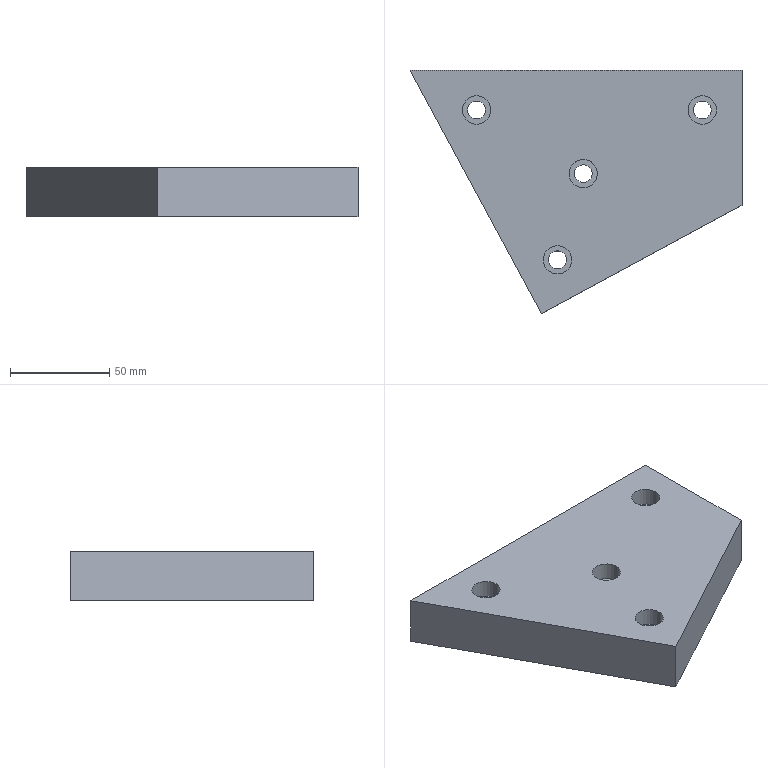Part | Creo | 1 solid | 26 faces | box 167.245 x 122.585 x 25 mm | volume 332373 mm3 | cylinder 16 | plane 10 | commonest cylinder face diameters 9 x8 14.25 x8
STEP:
#1=CARTESIAN_POINT('',(0.,0.,0.));
#2=DIRECTION('',(0.,0.,1.));
#3=DIRECTION('',(1.,0.,0.));
#4=AXIS2_PLACEMENT_3D('',#1,#2,#3);
#5=CARTESIAN_POINT('',(311.855,-89.244,-31.844));
#6=VERTEX_POINT('',#5);
#7=CARTESIAN_POINT('',(378.054,-211.829,-31.844));
#8=VERTEX_POINT('',#7);
#9=CARTESIAN_POINT('',(311.855,-89.244,-31.844));
#10=DIRECTION('',(0.4752,-0.8799,0.));
#11=VECTOR('',#10,139.317);
#12=LINE('',#9,#11);
#13=EDGE_CURVE('',#6,#8,#12,.T.);
#14=ORIENTED_EDGE('',*,*,#13,.F.);
#15=CARTESIAN_POINT('',(479.101,-89.244,-31.844));
#16=VERTEX_POINT('',#15);
#17=CARTESIAN_POINT('',(479.101,-89.244,-31.844));
#18=DIRECTION('',(-1.,0.,0.));
#19=VECTOR('',#18,167.245);
#20=LINE('',#17,#19);
#21=EDGE_CURVE('',#16,#6,#20,.T.);
#22=ORIENTED_EDGE('',*,*,#21,.F.);
#23=CARTESIAN_POINT('',(479.101,-157.262,-31.844));
#24=VERTEX_POINT('',#23);
#25=CARTESIAN_POINT('',(479.101,-89.244,-31.844));
#26=DIRECTION('',(0.,-1.,0.));
#27=VECTOR('',#26,68.018);
#28=LINE('',#25,#27);
#29=EDGE_CURVE('',#16,#24,#28,.T.);
#30=ORIENTED_EDGE('',*,*,#29,.T.);
#31=CARTESIAN_POINT('',(378.054,-211.829,-31.844));
#32=DIRECTION('',(0.8799,0.4752,0.));
#33=VECTOR('',#32,114.84);
#34=LINE('',#31,#33);
#35=EDGE_CURVE('',#8,#24,#34,.T.);
#36=ORIENTED_EDGE('',*,*,#35,.F.);
#37=EDGE_LOOP('',(#14,#22,#30,#36));
#38=FACE_OUTER_BOUND('',#37,.F.);
#39=CARTESIAN_POINT('',(338.261,-109.244,-31.844));
#40=VERTEX_POINT('',#39);
#41=CARTESIAN_POINT('',(352.511,-109.244,-31.844));
#42=VERTEX_POINT('',#41);
#43=CARTESIAN_POINT('',(345.386,-109.244,-31.844));
#44=DIRECTION('',(0.,0.,-1.));
#45=DIRECTION('',(-1.,0.,0.));
#46=AXIS2_PLACEMENT_3D('',#43,#44,#45);
#47=CIRCLE('',#46,7.125);
#48=EDGE_CURVE('',#40,#42,#47,.T.);
#49=ORIENTED_EDGE('',*,*,#48,.F.);
#50=CARTESIAN_POINT('',(345.386,-109.244,-31.844));
#51=DIRECTION('',(0.,0.,-1.));
#52=DIRECTION('',(1.,0.,0.));
#53=AXIS2_PLACEMENT_3D('',#50,#51,#52);
#54=CIRCLE('',#53,7.125);
#55=EDGE_CURVE('',#42,#40,#54,.T.);
#56=ORIENTED_EDGE('',*,*,#55,.F.);
#57=EDGE_LOOP('',(#49,#56));
#58=FACE_BOUND('',#57,.F.);
#59=CARTESIAN_POINT('',(451.976,-109.244,-31.844));
#60=VERTEX_POINT('',#59);
#61=CARTESIAN_POINT('',(466.226,-109.244,-31.844));
#62=VERTEX_POINT('',#61);
#63=CARTESIAN_POINT('',(459.101,-109.244,-31.844));
#64=DIRECTION('',(0.,0.,-1.));
#65=DIRECTION('',(-1.,0.,0.));
#66=AXIS2_PLACEMENT_3D('',#63,#64,#65);
#67=CIRCLE('',#66,7.125);
#68=EDGE_CURVE('',#60,#62,#67,.T.);
#69=ORIENTED_EDGE('',*,*,#68,.F.);
#70=CARTESIAN_POINT('',(459.101,-109.244,-31.844));
#71=DIRECTION('',(0.,0.,-1.));
#72=DIRECTION('',(1.,0.,0.));
#73=AXIS2_PLACEMENT_3D('',#70,#71,#72);
#74=CIRCLE('',#73,7.125);
#75=EDGE_CURVE('',#62,#60,#74,.T.);
#76=ORIENTED_EDGE('',*,*,#75,.F.);
#77=EDGE_LOOP('',(#69,#76));
#78=FACE_BOUND('',#77,.F.);
#79=CARTESIAN_POINT('',(391.996,-141.296,-31.844));
#80=VERTEX_POINT('',#79);
#81=CARTESIAN_POINT('',(406.246,-141.296,-31.844));
#82=VERTEX_POINT('',#81);
#83=CARTESIAN_POINT('',(399.121,-141.296,-31.844));
#84=DIRECTION('',(0.,0.,-1.));
#85=DIRECTION('',(-1.,0.,0.));
#86=AXIS2_PLACEMENT_3D('',#83,#84,#85);
#87=CIRCLE('',#86,7.125);
#88=EDGE_CURVE('',#80,#82,#87,.T.);
#89=ORIENTED_EDGE('',*,*,#88,.F.);
#90=CARTESIAN_POINT('',(399.121,-141.296,-31.844));
#91=DIRECTION('',(0.,0.,-1.));
#92=DIRECTION('',(1.,0.,0.));
#93=AXIS2_PLACEMENT_3D('',#90,#91,#92);
#94=CIRCLE('',#93,7.125);
#95=EDGE_CURVE('',#82,#80,#94,.T.);
#96=ORIENTED_EDGE('',*,*,#95,.F.);
#97=EDGE_LOOP('',(#89,#96));
#98=FACE_BOUND('',#97,.F.);
#99=CARTESIAN_POINT('',(379.023,-184.728,-31.844));
#100=VERTEX_POINT('',#99);
#101=CARTESIAN_POINT('',(393.273,-184.728,-31.844));
#102=VERTEX_POINT('',#101);
#103=CARTESIAN_POINT('',(386.148,-184.728,-31.844));
#104=DIRECTION('',(0.,0.,-1.));
#105=DIRECTION('',(-1.,0.,0.));
#106=AXIS2_PLACEMENT_3D('',#103,#104,#105);
#107=CIRCLE('',#106,7.125);
#108=EDGE_CURVE('',#100,#102,#107,.T.);
#109=ORIENTED_EDGE('',*,*,#108,.F.);
#110=CARTESIAN_POINT('',(386.148,-184.728,-31.844));
#111=DIRECTION('',(0.,0.,-1.));
#112=DIRECTION('',(1.,0.,0.));
#113=AXIS2_PLACEMENT_3D('',#110,#111,#112);
#114=CIRCLE('',#113,7.125);
#115=EDGE_CURVE('',#102,#100,#114,.T.);
#116=ORIENTED_EDGE('',*,*,#115,.F.);
#117=EDGE_LOOP('',(#109,#116));
#118=FACE_BOUND('',#117,.F.);
#119=CARTESIAN_POINT('',(356.671,-172.234,-31.844));
#120=DIRECTION('',(0.,0.,-1.));
#121=DIRECTION('',(-1.,0.,0.));
#122=AXIS2_PLACEMENT_3D('',#119,#120,#121);
#123=PLANE('',#122);
#124=ADVANCED_FACE('',(#38,#58,#78,#98,#118),#123,.F.);
#125=ORIENTED_EDGE('',*,*,#68,.T.);
#126=CARTESIAN_POINT('',(466.226,-109.244,-40.844));
#127=VERTEX_POINT('',#126);
#128=CARTESIAN_POINT('',(466.226,-109.244,-40.844));
#129=DIRECTION('',(0.,0.,1.));
#130=VECTOR('',#129,9.);
#131=LINE('',#128,#130);
#132=EDGE_CURVE('',#127,#62,#131,.T.);
#133=ORIENTED_EDGE('',*,*,#132,.F.);
#134=CARTESIAN_POINT('',(451.976,-109.244,-40.844));
#135=VERTEX_POINT('',#134);
#136=CARTESIAN_POINT('',(459.101,-109.244,-40.844));
#137=DIRECTION('',(0.,0.,1.));
#138=DIRECTION('',(1.,0.,0.));
#139=AXIS2_PLACEMENT_3D('',#136,#137,#138);
#140=CIRCLE('',#139,7.125);
#141=EDGE_CURVE('',#127,#135,#140,.T.);
#142=ORIENTED_EDGE('',*,*,#141,.T.);
#143=CARTESIAN_POINT('',(451.976,-109.244,-40.844));
#144=DIRECTION('',(0.,0.,1.));
#145=VECTOR('',#144,9.);
#146=LINE('',#143,#145);
#147=EDGE_CURVE('',#135,#60,#146,.T.);
#148=ORIENTED_EDGE('',*,*,#147,.T.);
#149=EDGE_LOOP('',(#125,#133,#142,#148));
#150=FACE_OUTER_BOUND('',#149,.F.);
#151=CARTESIAN_POINT('',(459.101,-109.244,-40.844));
#152=DIRECTION('',(0.,0.,1.));
#153=DIRECTION('',(1.,0.,0.));
#154=AXIS2_PLACEMENT_3D('',#151,#152,#153);
#155=CYLINDRICAL_SURFACE('',#154,7.125);
#156=ADVANCED_FACE('',(#150),#155,.F.);
#157=ORIENTED_EDGE('',*,*,#75,.T.);
#158=ORIENTED_EDGE('',*,*,#147,.F.);
#159=CARTESIAN_POINT('',(459.101,-109.244,-40.844));
#160=DIRECTION('',(0.,0.,1.));
#161=DIRECTION('',(-1.,0.,0.));
#162=AXIS2_PLACEMENT_3D('',#159,#160,#161);
#163=CIRCLE('',#162,7.125);
#164=EDGE_CURVE('',#135,#127,#163,.T.);
#165=ORIENTED_EDGE('',*,*,#164,.T.);
#166=ORIENTED_EDGE('',*,*,#132,.T.);
#167=EDGE_LOOP('',(#157,#158,#165,#166));
#168=FACE_OUTER_BOUND('',#167,.F.);
#169=CARTESIAN_POINT('',(459.101,-109.244,-40.844));
#170=DIRECTION('',(0.,0.,1.));
#171=DIRECTION('',(1.,0.,0.));
#172=AXIS2_PLACEMENT_3D('',#169,#170,#171);
#173=CYLINDRICAL_SURFACE('',#172,7.125);
#174=ADVANCED_FACE('',(#168),#173,.F.);
#175=ORIENTED_EDGE('',*,*,#164,.F.);
#176=ORIENTED_EDGE('',*,*,#141,.F.);
#177=EDGE_LOOP('',(#175,#176));
#178=FACE_OUTER_BOUND('',#177,.F.);
#179=CARTESIAN_POINT('',(463.601,-109.244,-40.844));
#180=VERTEX_POINT('',#179);
#181=CARTESIAN_POINT('',(454.601,-109.244,-40.844));
#182=VERTEX_POINT('',#181);
#183=CARTESIAN_POINT('',(459.101,-109.244,-40.844));
#184=DIRECTION('',(0.,0.,-1.));
#185=DIRECTION('',(1.,0.,0.));
#186=AXIS2_PLACEMENT_3D('',#183,#184,#185);
#187=CIRCLE('',#186,4.5);
#188=EDGE_CURVE('',#180,#182,#187,.T.);
#189=ORIENTED_EDGE('',*,*,#188,.F.);
#190=CARTESIAN_POINT('',(459.101,-109.244,-40.844));
#191=DIRECTION('',(0.,0.,-1.));
#192=DIRECTION('',(-1.,0.,0.));
#193=AXIS2_PLACEMENT_3D('',#190,#191,#192);
#194=CIRCLE('',#193,4.5);
#195=EDGE_CURVE('',#182,#180,#194,.T.);
#196=ORIENTED_EDGE('',*,*,#195,.F.);
#197=EDGE_LOOP('',(#189,#196));
#198=FACE_BOUND('',#197,.F.);
#199=CARTESIAN_POINT('',(459.101,-109.244,-40.844));
#200=DIRECTION('',(0.,0.,-1.));
#201=DIRECTION('',(-1.,0.,0.));
#202=AXIS2_PLACEMENT_3D('',#199,#200,#201);
#203=PLANE('',#202);
#204=ADVANCED_FACE('',(#178,#198),#203,.F.);
#205=CARTESIAN_POINT('',(454.601,-109.244,-56.844));
#206=VERTEX_POINT('',#205);
#207=CARTESIAN_POINT('',(463.601,-109.244,-56.844));
#208=VERTEX_POINT('',#207);
#209=CARTESIAN_POINT('',(459.101,-109.244,-56.844));
#210=DIRECTION('',(0.,0.,1.));
#211=DIRECTION('',(-1.,0.,0.));
#212=AXIS2_PLACEMENT_3D('',#209,#210,#211);
#213=CIRCLE('',#212,4.5);
#214=EDGE_CURVE('',#206,#208,#213,.T.);
#215=ORIENTED_EDGE('',*,*,#214,.T.);
#216=CARTESIAN_POINT('',(463.601,-109.244,-40.844));
#217=DIRECTION('',(0.,0.,-1.));
#218=VECTOR('',#217,16.);
#219=LINE('',#216,#218);
#220=EDGE_CURVE('',#180,#208,#219,.T.);
#221=ORIENTED_EDGE('',*,*,#220,.F.);
#222=ORIENTED_EDGE('',*,*,#188,.T.);
#223=CARTESIAN_POINT('',(454.601,-109.244,-40.844));
#224=DIRECTION('',(0.,0.,-1.));
#225=VECTOR('',#224,16.);
#226=LINE('',#223,#225);
#227=EDGE_CURVE('',#182,#206,#226,.T.);
#228=ORIENTED_EDGE('',*,*,#227,.T.);
#229=EDGE_LOOP('',(#215,#221,#222,#228));
#230=FACE_OUTER_BOUND('',#229,.F.);
#231=CARTESIAN_POINT('',(459.101,-109.244,-40.844));
#232=DIRECTION('',(0.,0.,-1.));
#233=DIRECTION('',(-1.,0.,0.));
#234=AXIS2_PLACEMENT_3D('',#231,#232,#233);
#235=CYLINDRICAL_SURFACE('',#234,4.5);
#236=ADVANCED_FACE('',(#230),#235,.F.);
#237=CARTESIAN_POINT('',(378.054,-211.829,-56.844));
#238=VERTEX_POINT('',#237);
#239=CARTESIAN_POINT('',(311.855,-89.244,-56.844));
#240=VERTEX_POINT('',#239);
#241=CARTESIAN_POINT('',(378.054,-211.829,-56.844));
#242=DIRECTION('',(-0.4752,0.8799,0.));
#243=VECTOR('',#242,139.317);
#244=LINE('',#241,#243);
#245=EDGE_CURVE('',#238,#240,#244,.T.);
#246=ORIENTED_EDGE('',*,*,#245,.F.);
#247=CARTESIAN_POINT('',(479.101,-157.262,-56.844));
#248=VERTEX_POINT('',#247);
#249=CARTESIAN_POINT('',(479.101,-157.262,-56.844));
#250=DIRECTION('',(-0.8799,-0.4752,0.));
#251=VECTOR('',#250,114.84);
#252=LINE('',#249,#251);
#253=EDGE_CURVE('',#248,#238,#252,.T.);
#254=ORIENTED_EDGE('',*,*,#253,.F.);
#255=CARTESIAN_POINT('',(479.101,-89.244,-56.844));
#256=VERTEX_POINT('',#255);
#257=CARTESIAN_POINT('',(479.101,-89.244,-56.844));
#258=DIRECTION('',(0.,-1.,0.));
#259=VECTOR('',#258,68.018);
#260=LINE('',#257,#259);
#261=EDGE_CURVE('',#256,#248,#260,.T.);
#262=ORIENTED_EDGE('',*,*,#261,.F.);
#263=CARTESIAN_POINT('',(479.101,-89.244,-56.844));
#264=DIRECTION('',(-1.,0.,0.));
#265=VECTOR('',#264,167.245);
#266=LINE('',#263,#265);
#267=EDGE_CURVE('',#256,#240,#266,.T.);
#268=ORIENTED_EDGE('',*,*,#267,.T.);
#269=EDGE_LOOP('',(#246,#254,#262,#268));
#270=FACE_OUTER_BOUND('',#269,.F.);
#271=CARTESIAN_POINT('',(459.101,-109.244,-56.844));
#272=DIRECTION('',(0.,0.,1.));
#273=DIRECTION('',(1.,0.,0.));
#274=AXIS2_PLACEMENT_3D('',#271,#272,#273);
#275=CIRCLE('',#274,4.5);
#276=EDGE_CURVE('',#208,#206,#275,.T.);
#277=ORIENTED_EDGE('',*,*,#276,.F.);
#278=ORIENTED_EDGE('',*,*,#214,.F.);
#279=EDGE_LOOP('',(#277,#278));
#280=FACE_BOUND('',#279,.F.);
#281=CARTESIAN_POINT('',(403.621,-141.296,-56.844));
#282=VERTEX_POINT('',#281);
#283=CARTESIAN_POINT('',(394.621,-141.296,-56.844));
#284=VERTEX_POINT('',#283);
#285=CARTESIAN_POINT('',(399.121,-141.296,-56.844));
#286=DIRECTION('',(0.,0.,1.));
#287=DIRECTION('',(1.,0.,0.));
#288=AXIS2_PLACEMENT_3D('',#285,#286,#287);
#289=CIRCLE('',#288,4.5);
#290=EDGE_CURVE('',#282,#284,#289,.T.);
#291=ORIENTED_EDGE('',*,*,#290,.F.);
#292=CARTESIAN_POINT('',(399.121,-141.296,-56.844));
#293=DIRECTION('',(0.,0.,1.));
#294=DIRECTION('',(-1.,0.,0.));
#295=AXIS2_PLACEMENT_3D('',#292,#293,#294);
#296=CIRCLE('',#295,4.5);
#297=EDGE_CURVE('',#284,#282,#296,.T.);
#298=ORIENTED_EDGE('',*,*,#297,.F.);
#299=EDGE_LOOP('',(#291,#298));
#300=FACE_BOUND('',#299,.F.);
#301=CARTESIAN_POINT('',(349.886,-109.244,-56.844));
#302=VERTEX_POINT('',#301);
#303=CARTESIAN_POINT('',(340.886,-109.244,-56.844));
#304=VERTEX_POINT('',#303);
#305=CARTESIAN_POINT('',(345.386,-109.244,-56.844));
#306=DIRECTION('',(0.,0.,1.));
#307=DIRECTION('',(1.,0.,0.));
#308=AXIS2_PLACEMENT_3D('',#305,#306,#307);
#309=CIRCLE('',#308,4.5);
#310=EDGE_CURVE('',#302,#304,#309,.T.);
#311=ORIENTED_EDGE('',*,*,#310,.F.);
#312=CARTESIAN_POINT('',(345.386,-109.244,-56.844));
#313=DIRECTION('',(0.,0.,1.));
#314=DIRECTION('',(-1.,0.,0.));
#315=AXIS2_PLACEMENT_3D('',#312,#313,#314);
#316=CIRCLE('',#315,4.5);
#317=EDGE_CURVE('',#304,#302,#316,.T.);
#318=ORIENTED_EDGE('',*,*,#317,.F.);
#319=EDGE_LOOP('',(#311,#318));
#320=FACE_BOUND('',#319,.F.);
#321=CARTESIAN_POINT('',(390.648,-184.728,-56.844));
#322=VERTEX_POINT('',#321);
#323=CARTESIAN_POINT('',(381.648,-184.728,-56.844));
#324=VERTEX_POINT('',#323);
#325=CARTESIAN_POINT('',(386.148,-184.728,-56.844));
#326=DIRECTION('',(0.,0.,1.));
#327=DIRECTION('',(1.,0.,0.));
#328=AXIS2_PLACEMENT_3D('',#325,#326,#327);
#329=CIRCLE('',#328,4.5);
#330=EDGE_CURVE('',#322,#324,#329,.T.);
#331=ORIENTED_EDGE('',*,*,#330,.F.);
#332=CARTESIAN_POINT('',(386.148,-184.728,-56.844));
#333=DIRECTION('',(0.,0.,1.));
#334=DIRECTION('',(-1.,0.,0.));
#335=AXIS2_PLACEMENT_3D('',#332,#333,#334);
#336=CIRCLE('',#335,4.5);
#337=EDGE_CURVE('',#324,#322,#336,.T.);
#338=ORIENTED_EDGE('',*,*,#337,.F.);
#339=EDGE_LOOP('',(#331,#338));
#340=FACE_BOUND('',#339,.F.);
#341=CARTESIAN_POINT('',(356.671,-172.234,-56.844));
#342=DIRECTION('',(0.,0.,-1.));
#343=DIRECTION('',(-1.,0.,0.));
#344=AXIS2_PLACEMENT_3D('',#341,#342,#343);
#345=PLANE('',#344);
#346=ADVANCED_FACE('',(#270,#280,#300,#320,#340),#345,.T.);
#347=ORIENTED_EDGE('',*,*,#330,.T.);
#348=CARTESIAN_POINT('',(381.648,-184.728,-40.844));
#349=VERTEX_POINT('',#348);
#350=CARTESIAN_POINT('',(381.648,-184.728,-40.844));
#351=DIRECTION('',(0.,0.,-1.));
#352=VECTOR('',#351,16.);
#353=LINE('',#350,#352);
#354=EDGE_CURVE('',#349,#324,#353,.T.);
#355=ORIENTED_EDGE('',*,*,#354,.F.);
#356=CARTESIAN_POINT('',(390.648,-184.728,-40.844));
#357=VERTEX_POINT('',#356);
#358=CARTESIAN_POINT('',(386.148,-184.728,-40.844));
#359=DIRECTION('',(0.,0.,-1.));
#360=DIRECTION('',(-1.,0.,0.));
#361=AXIS2_PLACEMENT_3D('',#358,#359,#360);
#362=CIRCLE('',#361,4.5);
#363=EDGE_CURVE('',#349,#357,#362,.T.);
#364=ORIENTED_EDGE('',*,*,#363,.T.);
#365=CARTESIAN_POINT('',(390.648,-184.728,-40.844));
#366=DIRECTION('',(0.,0.,-1.));
#367=VECTOR('',#366,16.);
#368=LINE('',#365,#367);
#369=EDGE_CURVE('',#357,#322,#368,.T.);
#370=ORIENTED_EDGE('',*,*,#369,.T.);
#371=EDGE_LOOP('',(#347,#355,#364,#370));
#372=FACE_OUTER_BOUND('',#371,.F.);
#373=CARTESIAN_POINT('',(386.148,-184.728,-40.844));
#374=DIRECTION('',(0.,0.,-1.));
#375=DIRECTION('',(-1.,0.,0.));
#376=AXIS2_PLACEMENT_3D('',#373,#374,#375);
#377=CYLINDRICAL_SURFACE('',#376,4.5);
#378=ADVANCED_FACE('',(#372),#377,.F.);
#379=ORIENTED_EDGE('',*,*,#337,.T.);
#380=ORIENTED_EDGE('',*,*,#369,.F.);
#381=CARTESIAN_POINT('',(386.148,-184.728,-40.844));
#382=DIRECTION('',(0.,0.,-1.));
#383=DIRECTION('',(1.,0.,0.));
#384=AXIS2_PLACEMENT_3D('',#381,#382,#383);
#385=CIRCLE('',#384,4.5);
#386=EDGE_CURVE('',#357,#349,#385,.T.);
#387=ORIENTED_EDGE('',*,*,#386,.T.);
#388=ORIENTED_EDGE('',*,*,#354,.T.);
#389=EDGE_LOOP('',(#379,#380,#387,#388));
#390=FACE_OUTER_BOUND('',#389,.F.);
#391=CARTESIAN_POINT('',(386.148,-184.728,-40.844));
#392=DIRECTION('',(0.,0.,-1.));
#393=DIRECTION('',(-1.,0.,0.));
#394=AXIS2_PLACEMENT_3D('',#391,#392,#393);
#395=CYLINDRICAL_SURFACE('',#394,4.5);
#396=ADVANCED_FACE('',(#390),#395,.F.);
#397=CARTESIAN_POINT('',(379.023,-184.728,-40.844));
#398=VERTEX_POINT('',#397);
#399=CARTESIAN_POINT('',(393.273,-184.728,-40.844));
#400=VERTEX_POINT('',#399);
#401=CARTESIAN_POINT('',(386.148,-184.728,-40.844));
#402=DIRECTION('',(0.,0.,1.));
#403=DIRECTION('',(-1.,0.,0.));
#404=AXIS2_PLACEMENT_3D('',#401,#402,#403);
#405=CIRCLE('',#404,7.125);
#406=EDGE_CURVE('',#398,#400,#405,.T.);
#407=ORIENTED_EDGE('',*,*,#406,.F.);
#408=CARTESIAN_POINT('',(386.148,-184.728,-40.844));
#409=DIRECTION('',(0.,0.,1.));
#410=DIRECTION('',(1.,0.,0.));
#411=AXIS2_PLACEMENT_3D('',#408,#409,#410);
#412=CIRCLE('',#411,7.125);
#413=EDGE_CURVE('',#400,#398,#412,.T.);
#414=ORIENTED_EDGE('',*,*,#413,.F.);
#415=EDGE_LOOP('',(#407,#414));
#416=FACE_OUTER_BOUND('',#415,.F.);
#417=ORIENTED_EDGE('',*,*,#386,.F.);
#418=ORIENTED_EDGE('',*,*,#363,.F.);
#419=EDGE_LOOP('',(#417,#418));
#420=FACE_BOUND('',#419,.F.);
#421=CARTESIAN_POINT('',(386.148,-184.728,-40.844));
#422=DIRECTION('',(0.,0.,-1.));
#423=DIRECTION('',(-1.,0.,0.));
#424=AXIS2_PLACEMENT_3D('',#421,#422,#423);
#425=PLANE('',#424);
#426=ADVANCED_FACE('',(#416,#420),#425,.F.);
#427=ORIENTED_EDGE('',*,*,#115,.T.);
#428=CARTESIAN_POINT('',(379.023,-184.728,-40.844));
#429=DIRECTION('',(0.,0.,1.));
#430=VECTOR('',#429,9.);
#431=LINE('',#428,#430);
#432=EDGE_CURVE('',#398,#100,#431,.T.);
#433=ORIENTED_EDGE('',*,*,#432,.F.);
#434=ORIENTED_EDGE('',*,*,#406,.T.);
#435=CARTESIAN_POINT('',(393.273,-184.728,-40.844));
#436=DIRECTION('',(0.,0.,1.));
#437=VECTOR('',#436,9.);
#438=LINE('',#435,#437);
#439=EDGE_CURVE('',#400,#102,#438,.T.);
#440=ORIENTED_EDGE('',*,*,#439,.T.);
#441=EDGE_LOOP('',(#427,#433,#434,#440));
#442=FACE_OUTER_BOUND('',#441,.F.);
#443=CARTESIAN_POINT('',(386.148,-184.728,-40.844));
#444=DIRECTION('',(0.,0.,1.));
#445=DIRECTION('',(1.,0.,0.));
#446=AXIS2_PLACEMENT_3D('',#443,#444,#445);
#447=CYLINDRICAL_SURFACE('',#446,7.125);
#448=ADVANCED_FACE('',(#442),#447,.F.);
#449=ORIENTED_EDGE('',*,*,#108,.T.);
#450=ORIENTED_EDGE('',*,*,#439,.F.);
#451=ORIENTED_EDGE('',*,*,#413,.T.);
#452=ORIENTED_EDGE('',*,*,#432,.T.);
#453=EDGE_LOOP('',(#449,#450,#451,#452));
#454=FACE_OUTER_BOUND('',#453,.F.);
#455=CARTESIAN_POINT('',(386.148,-184.728,-40.844));
#456=DIRECTION('',(0.,0.,1.));
#457=DIRECTION('',(1.,0.,0.));
#458=AXIS2_PLACEMENT_3D('',#455,#456,#457);
#459=CYLINDRICAL_SURFACE('',#458,7.125);
#460=ADVANCED_FACE('',(#454),#459,.F.);
#461=ORIENTED_EDGE('',*,*,#276,.T.);
#462=ORIENTED_EDGE('',*,*,#227,.F.);
#463=ORIENTED_EDGE('',*,*,#195,.T.);
#464=ORIENTED_EDGE('',*,*,#220,.T.);
#465=EDGE_LOOP('',(#461,#462,#463,#464));
#466=FACE_OUTER_BOUND('',#465,.F.);
#467=CARTESIAN_POINT('',(459.101,-109.244,-40.844));
#468=DIRECTION('',(0.,0.,-1.));
#469=DIRECTION('',(-1.,0.,0.));
#470=AXIS2_PLACEMENT_3D('',#467,#468,#469);
#471=CYLINDRICAL_SURFACE('',#470,4.5);
#472=ADVANCED_FACE('',(#466),#471,.F.);
#473=ORIENTED_EDGE('',*,*,#290,.T.);
#474=CARTESIAN_POINT('',(394.621,-141.296,-40.844));
#475=VERTEX_POINT('',#474);
#476=CARTESIAN_POINT('',(394.621,-141.296,-40.844));
#477=DIRECTION('',(0.,0.,-1.));
#478=VECTOR('',#477,16.);
#479=LINE('',#476,#478);
#480=EDGE_CURVE('',#475,#284,#479,.T.);
#481=ORIENTED_EDGE('',*,*,#480,.F.);
#482=CARTESIAN_POINT('',(403.621,-141.296,-40.844));
#483=VERTEX_POINT('',#482);
#484=CARTESIAN_POINT('',(399.121,-141.296,-40.844));
#485=DIRECTION('',(0.,0.,-1.));
#486=DIRECTION('',(-1.,0.,0.));
#487=AXIS2_PLACEMENT_3D('',#484,#485,#486);
#488=CIRCLE('',#487,4.5);
#489=EDGE_CURVE('',#475,#483,#488,.T.);
#490=ORIENTED_EDGE('',*,*,#489,.T.);
#491=CARTESIAN_POINT('',(403.621,-141.296,-40.844));
#492=DIRECTION('',(0.,0.,-1.));
#493=VECTOR('',#492,16.);
#494=LINE('',#491,#493);
#495=EDGE_CURVE('',#483,#282,#494,.T.);
#496=ORIENTED_EDGE('',*,*,#495,.T.);
#497=EDGE_LOOP('',(#473,#481,#490,#496));
#498=FACE_OUTER_BOUND('',#497,.F.);
#499=CARTESIAN_POINT('',(399.121,-141.296,-40.844));
#500=DIRECTION('',(0.,0.,-1.));
#501=DIRECTION('',(-1.,0.,0.));
#502=AXIS2_PLACEMENT_3D('',#499,#500,#501);
#503=CYLINDRICAL_SURFACE('',#502,4.5);
#504=ADVANCED_FACE('',(#498),#503,.F.);
#505=ORIENTED_EDGE('',*,*,#297,.T.);
#506=ORIENTED_EDGE('',*,*,#495,.F.);
#507=CARTESIAN_POINT('',(399.121,-141.296,-40.844));
#508=DIRECTION('',(0.,0.,-1.));
#509=DIRECTION('',(1.,0.,0.));
#510=AXIS2_PLACEMENT_3D('',#507,#508,#509);
#511=CIRCLE('',#510,4.5);
#512=EDGE_CURVE('',#483,#475,#511,.T.);
#513=ORIENTED_EDGE('',*,*,#512,.T.);
#514=ORIENTED_EDGE('',*,*,#480,.T.);
#515=EDGE_LOOP('',(#505,#506,#513,#514));
#516=FACE_OUTER_BOUND('',#515,.F.);
#517=CARTESIAN_POINT('',(399.121,-141.296,-40.844));
#518=DIRECTION('',(0.,0.,-1.));
#519=DIRECTION('',(-1.,0.,0.));
#520=AXIS2_PLACEMENT_3D('',#517,#518,#519);
#521=CYLINDRICAL_SURFACE('',#520,4.5);
#522=ADVANCED_FACE('',(#516),#521,.F.);
#523=CARTESIAN_POINT('',(391.996,-141.296,-40.844));
#524=VERTEX_POINT('',#523);
#525=CARTESIAN_POINT('',(406.246,-141.296,-40.844));
#526=VERTEX_POINT('',#525);
#527=CARTESIAN_POINT('',(399.121,-141.296,-40.844));
#528=DIRECTION('',(0.,0.,1.));
#529=DIRECTION('',(-1.,0.,0.));
#530=AXIS2_PLACEMENT_3D('',#527,#528,#529);
#531=CIRCLE('',#530,7.125);
#532=EDGE_CURVE('',#524,#526,#531,.T.);
#533=ORIENTED_EDGE('',*,*,#532,.F.);
#534=CARTESIAN_POINT('',(399.121,-141.296,-40.844));
#535=DIRECTION('',(0.,0.,1.));
#536=DIRECTION('',(1.,0.,0.));
#537=AXIS2_PLACEMENT_3D('',#534,#535,#536);
#538=CIRCLE('',#537,7.125);
#539=EDGE_CURVE('',#526,#524,#538,.T.);
#540=ORIENTED_EDGE('',*,*,#539,.F.);
#541=EDGE_LOOP('',(#533,#540));
#542=FACE_OUTER_BOUND('',#541,.F.);
#543=ORIENTED_EDGE('',*,*,#512,.F.);
#544=ORIENTED_EDGE('',*,*,#489,.F.);
#545=EDGE_LOOP('',(#543,#544));
#546=FACE_BOUND('',#545,.F.);
#547=CARTESIAN_POINT('',(399.121,-141.296,-40.844));
#548=DIRECTION('',(0.,0.,-1.));
#549=DIRECTION('',(-1.,0.,0.));
#550=AXIS2_PLACEMENT_3D('',#547,#548,#549);
#551=PLANE('',#550);
#552=ADVANCED_FACE('',(#542,#546),#551,.F.);
#553=ORIENTED_EDGE('',*,*,#95,.T.);
#554=CARTESIAN_POINT('',(391.996,-141.296,-40.844));
#555=DIRECTION('',(0.,0.,1.));
#556=VECTOR('',#555,9.);
#557=LINE('',#554,#556);
#558=EDGE_CURVE('',#524,#80,#557,.T.);
#559=ORIENTED_EDGE('',*,*,#558,.F.);
#560=ORIENTED_EDGE('',*,*,#532,.T.);
#561=CARTESIAN_POINT('',(406.246,-141.296,-40.844));
#562=DIRECTION('',(0.,0.,1.));
#563=VECTOR('',#562,9.);
#564=LINE('',#561,#563);
#565=EDGE_CURVE('',#526,#82,#564,.T.);
#566=ORIENTED_EDGE('',*,*,#565,.T.);
#567=EDGE_LOOP('',(#553,#559,#560,#566));
#568=FACE_OUTER_BOUND('',#567,.F.);
#569=CARTESIAN_POINT('',(399.121,-141.296,-40.844));
#570=DIRECTION('',(0.,0.,1.));
#571=DIRECTION('',(1.,0.,0.));
#572=AXIS2_PLACEMENT_3D('',#569,#570,#571);
#573=CYLINDRICAL_SURFACE('',#572,7.125);
#574=ADVANCED_FACE('',(#568),#573,.F.);
#575=ORIENTED_EDGE('',*,*,#88,.T.);
#576=ORIENTED_EDGE('',*,*,#565,.F.);
#577=ORIENTED_EDGE('',*,*,#539,.T.);
#578=ORIENTED_EDGE('',*,*,#558,.T.);
#579=EDGE_LOOP('',(#575,#576,#577,#578));
#580=FACE_OUTER_BOUND('',#579,.F.);
#581=CARTESIAN_POINT('',(399.121,-141.296,-40.844));
#582=DIRECTION('',(0.,0.,1.));
#583=DIRECTION('',(1.,0.,0.));
#584=AXIS2_PLACEMENT_3D('',#581,#582,#583);
#585=CYLINDRICAL_SURFACE('',#584,7.125);
#586=ADVANCED_FACE('',(#580),#585,.F.);
#587=ORIENTED_EDGE('',*,*,#310,.T.);
#588=CARTESIAN_POINT('',(340.886,-109.244,-40.844));
#589=VERTEX_POINT('',#588);
#590=CARTESIAN_POINT('',(340.886,-109.244,-40.844));
#591=DIRECTION('',(0.,0.,-1.));
#592=VECTOR('',#591,16.);
#593=LINE('',#590,#592);
#594=EDGE_CURVE('',#589,#304,#593,.T.);
#595=ORIENTED_EDGE('',*,*,#594,.F.);
#596=CARTESIAN_POINT('',(349.886,-109.244,-40.844));
#597=VERTEX_POINT('',#596);
#598=CARTESIAN_POINT('',(345.386,-109.244,-40.844));
#599=DIRECTION('',(0.,0.,-1.));
#600=DIRECTION('',(-1.,0.,0.));
#601=AXIS2_PLACEMENT_3D('',#598,#599,#600);
#602=CIRCLE('',#601,4.5);
#603=EDGE_CURVE('',#589,#597,#602,.T.);
#604=ORIENTED_EDGE('',*,*,#603,.T.);
#605=CARTESIAN_POINT('',(349.886,-109.244,-40.844));
#606=DIRECTION('',(0.,0.,-1.));
#607=VECTOR('',#606,16.);
#608=LINE('',#605,#607);
#609=EDGE_CURVE('',#597,#302,#608,.T.);
#610=ORIENTED_EDGE('',*,*,#609,.T.);
#611=EDGE_LOOP('',(#587,#595,#604,#610));
#612=FACE_OUTER_BOUND('',#611,.F.);
#613=CARTESIAN_POINT('',(345.386,-109.244,-40.844));
#614=DIRECTION('',(0.,0.,-1.));
#615=DIRECTION('',(-1.,0.,0.));
#616=AXIS2_PLACEMENT_3D('',#613,#614,#615);
#617=CYLINDRICAL_SURFACE('',#616,4.5);
#618=ADVANCED_FACE('',(#612),#617,.F.);
#619=ORIENTED_EDGE('',*,*,#317,.T.);
#620=ORIENTED_EDGE('',*,*,#609,.F.);
#621=CARTESIAN_POINT('',(345.386,-109.244,-40.844));
#622=DIRECTION('',(0.,0.,-1.));
#623=DIRECTION('',(1.,0.,0.));
#624=AXIS2_PLACEMENT_3D('',#621,#622,#623);
#625=CIRCLE('',#624,4.5);
#626=EDGE_CURVE('',#597,#589,#625,.T.);
#627=ORIENTED_EDGE('',*,*,#626,.T.);
#628=ORIENTED_EDGE('',*,*,#594,.T.);
#629=EDGE_LOOP('',(#619,#620,#627,#628));
#630=FACE_OUTER_BOUND('',#629,.F.);
#631=CARTESIAN_POINT('',(345.386,-109.244,-40.844));
#632=DIRECTION('',(0.,0.,-1.));
#633=DIRECTION('',(-1.,0.,0.));
#634=AXIS2_PLACEMENT_3D('',#631,#632,#633);
#635=CYLINDRICAL_SURFACE('',#634,4.5);
#636=ADVANCED_FACE('',(#630),#635,.F.);
#637=CARTESIAN_POINT('',(338.261,-109.244,-40.844));
#638=VERTEX_POINT('',#637);
#639=CARTESIAN_POINT('',(352.511,-109.244,-40.844));
#640=VERTEX_POINT('',#639);
#641=CARTESIAN_POINT('',(345.386,-109.244,-40.844));
#642=DIRECTION('',(0.,0.,1.));
#643=DIRECTION('',(-1.,0.,0.));
#644=AXIS2_PLACEMENT_3D('',#641,#642,#643);
#645=CIRCLE('',#644,7.125);
#646=EDGE_CURVE('',#638,#640,#645,.T.);
#647=ORIENTED_EDGE('',*,*,#646,.F.);
#648=CARTESIAN_POINT('',(345.386,-109.244,-40.844));
#649=DIRECTION('',(0.,0.,1.));
#650=DIRECTION('',(1.,0.,0.));
#651=AXIS2_PLACEMENT_3D('',#648,#649,#650);
#652=CIRCLE('',#651,7.125);
#653=EDGE_CURVE('',#640,#638,#652,.T.);
#654=ORIENTED_EDGE('',*,*,#653,.F.);
#655=EDGE_LOOP('',(#647,#654));
#656=FACE_OUTER_BOUND('',#655,.F.);
#657=ORIENTED_EDGE('',*,*,#626,.F.);
#658=ORIENTED_EDGE('',*,*,#603,.F.);
#659=EDGE_LOOP('',(#657,#658));
#660=FACE_BOUND('',#659,.F.);
#661=CARTESIAN_POINT('',(345.386,-109.244,-40.844));
#662=DIRECTION('',(0.,0.,-1.));
#663=DIRECTION('',(-1.,0.,0.));
#664=AXIS2_PLACEMENT_3D('',#661,#662,#663);
#665=PLANE('',#664);
#666=ADVANCED_FACE('',(#656,#660),#665,.F.);
#667=ORIENTED_EDGE('',*,*,#55,.T.);
#668=CARTESIAN_POINT('',(338.261,-109.244,-40.844));
#669=DIRECTION('',(0.,0.,1.));
#670=VECTOR('',#669,9.);
#671=LINE('',#668,#670);
#672=EDGE_CURVE('',#638,#40,#671,.T.);
#673=ORIENTED_EDGE('',*,*,#672,.F.);
#674=ORIENTED_EDGE('',*,*,#646,.T.);
#675=CARTESIAN_POINT('',(352.511,-109.244,-40.844));
#676=DIRECTION('',(0.,0.,1.));
#677=VECTOR('',#676,9.);
#678=LINE('',#675,#677);
#679=EDGE_CURVE('',#640,#42,#678,.T.);
#680=ORIENTED_EDGE('',*,*,#679,.T.);
#681=EDGE_LOOP('',(#667,#673,#674,#680));
#682=FACE_OUTER_BOUND('',#681,.F.);
#683=CARTESIAN_POINT('',(345.386,-109.244,-40.844));
#684=DIRECTION('',(0.,0.,1.));
#685=DIRECTION('',(1.,0.,0.));
#686=AXIS2_PLACEMENT_3D('',#683,#684,#685);
#687=CYLINDRICAL_SURFACE('',#686,7.125);
#688=ADVANCED_FACE('',(#682),#687,.F.);
#689=ORIENTED_EDGE('',*,*,#48,.T.);
#690=ORIENTED_EDGE('',*,*,#679,.F.);
#691=ORIENTED_EDGE('',*,*,#653,.T.);
#692=ORIENTED_EDGE('',*,*,#672,.T.);
#693=EDGE_LOOP('',(#689,#690,#691,#692));
#694=FACE_OUTER_BOUND('',#693,.F.);
#695=CARTESIAN_POINT('',(345.386,-109.244,-40.844));
#696=DIRECTION('',(0.,0.,1.));
#697=DIRECTION('',(1.,0.,0.));
#698=AXIS2_PLACEMENT_3D('',#695,#696,#697);
#699=CYLINDRICAL_SURFACE('',#698,7.125);
#700=ADVANCED_FACE('',(#694),#699,.F.);
#701=ORIENTED_EDGE('',*,*,#245,.T.);
#702=CARTESIAN_POINT('',(311.855,-89.244,-56.844));
#703=DIRECTION('',(0.,0.,1.));
#704=VECTOR('',#703,25.);
#705=LINE('',#702,#704);
#706=EDGE_CURVE('',#240,#6,#705,.T.);
#707=ORIENTED_EDGE('',*,*,#706,.T.);
#708=ORIENTED_EDGE('',*,*,#13,.T.);
#709=CARTESIAN_POINT('',(378.054,-211.829,-56.844));
#710=DIRECTION('',(0.,0.,1.));
#711=VECTOR('',#710,25.);
#712=LINE('',#709,#711);
#713=EDGE_CURVE('',#238,#8,#712,.T.);
#714=ORIENTED_EDGE('',*,*,#713,.F.);
#715=EDGE_LOOP('',(#701,#707,#708,#714));
#716=FACE_OUTER_BOUND('',#715,.F.);
#717=CARTESIAN_POINT('',(356.671,-172.234,-66.844));
#718=DIRECTION('',(0.8799,0.4752,0.));
#719=DIRECTION('',(-0.4752,0.8799,0.));
#720=AXIS2_PLACEMENT_3D('',#717,#718,#719);
#721=PLANE('',#720);
#722=ADVANCED_FACE('',(#716),#721,.F.);
#723=ORIENTED_EDGE('',*,*,#267,.F.);
#724=CARTESIAN_POINT('',(479.101,-89.244,-56.844));
#725=DIRECTION('',(0.,0.,1.));
#726=VECTOR('',#725,25.);
#727=LINE('',#724,#726);
#728=EDGE_CURVE('',#256,#16,#727,.T.);
#729=ORIENTED_EDGE('',*,*,#728,.T.);
#730=ORIENTED_EDGE('',*,*,#21,.T.);
#731=ORIENTED_EDGE('',*,*,#706,.F.);
#732=EDGE_LOOP('',(#723,#729,#730,#731));
#733=FACE_OUTER_BOUND('',#732,.F.);
#734=CARTESIAN_POINT('',(387.601,-89.244,-92.96));
#735=DIRECTION('',(0.,-1.,0.));
#736=DIRECTION('',(0.,0.,-1.));
#737=AXIS2_PLACEMENT_3D('',#734,#735,#736);
#738=PLANE('',#737);
#739=ADVANCED_FACE('',(#733),#738,.F.);
#740=ORIENTED_EDGE('',*,*,#261,.T.);
#741=CARTESIAN_POINT('',(479.101,-157.262,-56.844));
#742=DIRECTION('',(0.,0.,1.));
#743=VECTOR('',#742,25.);
#744=LINE('',#741,#743);
#745=EDGE_CURVE('',#248,#24,#744,.T.);
#746=ORIENTED_EDGE('',*,*,#745,.T.);
#747=ORIENTED_EDGE('',*,*,#29,.F.);
#748=ORIENTED_EDGE('',*,*,#728,.F.);
#749=EDGE_LOOP('',(#740,#746,#747,#748));
#750=FACE_OUTER_BOUND('',#749,.F.);
#751=CARTESIAN_POINT('',(479.101,250.373,-228.441));
#752=DIRECTION('',(-1.,0.,0.));
#753=DIRECTION('',(0.,-1.,0.));
#754=AXIS2_PLACEMENT_3D('',#751,#752,#753);
#755=PLANE('',#754);
#756=ADVANCED_FACE('',(#750),#755,.F.);
#757=ORIENTED_EDGE('',*,*,#253,.T.);
#758=ORIENTED_EDGE('',*,*,#713,.T.);
#759=ORIENTED_EDGE('',*,*,#35,.T.);
#760=ORIENTED_EDGE('',*,*,#745,.F.);
#761=EDGE_LOOP('',(#757,#758,#759,#760));
#762=FACE_OUTER_BOUND('',#761,.F.);
#763=CARTESIAN_POINT('',(378.054,-211.829,-66.844));
#764=DIRECTION('',(0.4752,-0.8799,0.));
#765=DIRECTION('',(0.8799,0.4752,0.));
#766=AXIS2_PLACEMENT_3D('',#763,#764,#765);
#767=PLANE('',#766);
#768=ADVANCED_FACE('',(#762),#767,.T.);
#769=CLOSED_SHELL('',(#124,#156,#174,#204,#236,#346,#378,#396,#426,#448,#460,#472,#504,#522,#552,#574,#586,#618,#636,#666,#688,#700,#722,#739,#756,#768));
#770=MANIFOLD_SOLID_BREP('',#769);
#771=(LENGTH_UNIT()NAMED_UNIT(*)SI_UNIT(.MILLI.,.METRE.));
#772=UNCERTAINTY_MEASURE_WITH_UNIT(LENGTH_MEASURE(0.02089),#771,'','');
#773=(NAMED_UNIT(*)PLANE_ANGLE_UNIT()SI_UNIT($,.RADIAN.));
#774=PLANE_ANGLE_MEASURE_WITH_UNIT(PLANE_ANGLE_MEASURE(0.01745),#773);
#775=(CONVERSION_BASED_UNIT('DEGREE',#774)NAMED_UNIT(*)PLANE_ANGLE_UNIT());
#776=(NAMED_UNIT(*)SI_UNIT($,.STERADIAN.)SOLID_ANGLE_UNIT());
#777=(GEOMETRIC_REPRESENTATION_CONTEXT(3)GLOBAL_UNCERTAINTY_ASSIGNED_CONTEXT((#772))GLOBAL_UNIT_ASSIGNED_CONTEXT((#771,#775,#776))REPRESENTATION_CONTEXT('',''));
#778=ADVANCED_BREP_SHAPE_REPRESENTATION('',(#4,#770),#777);